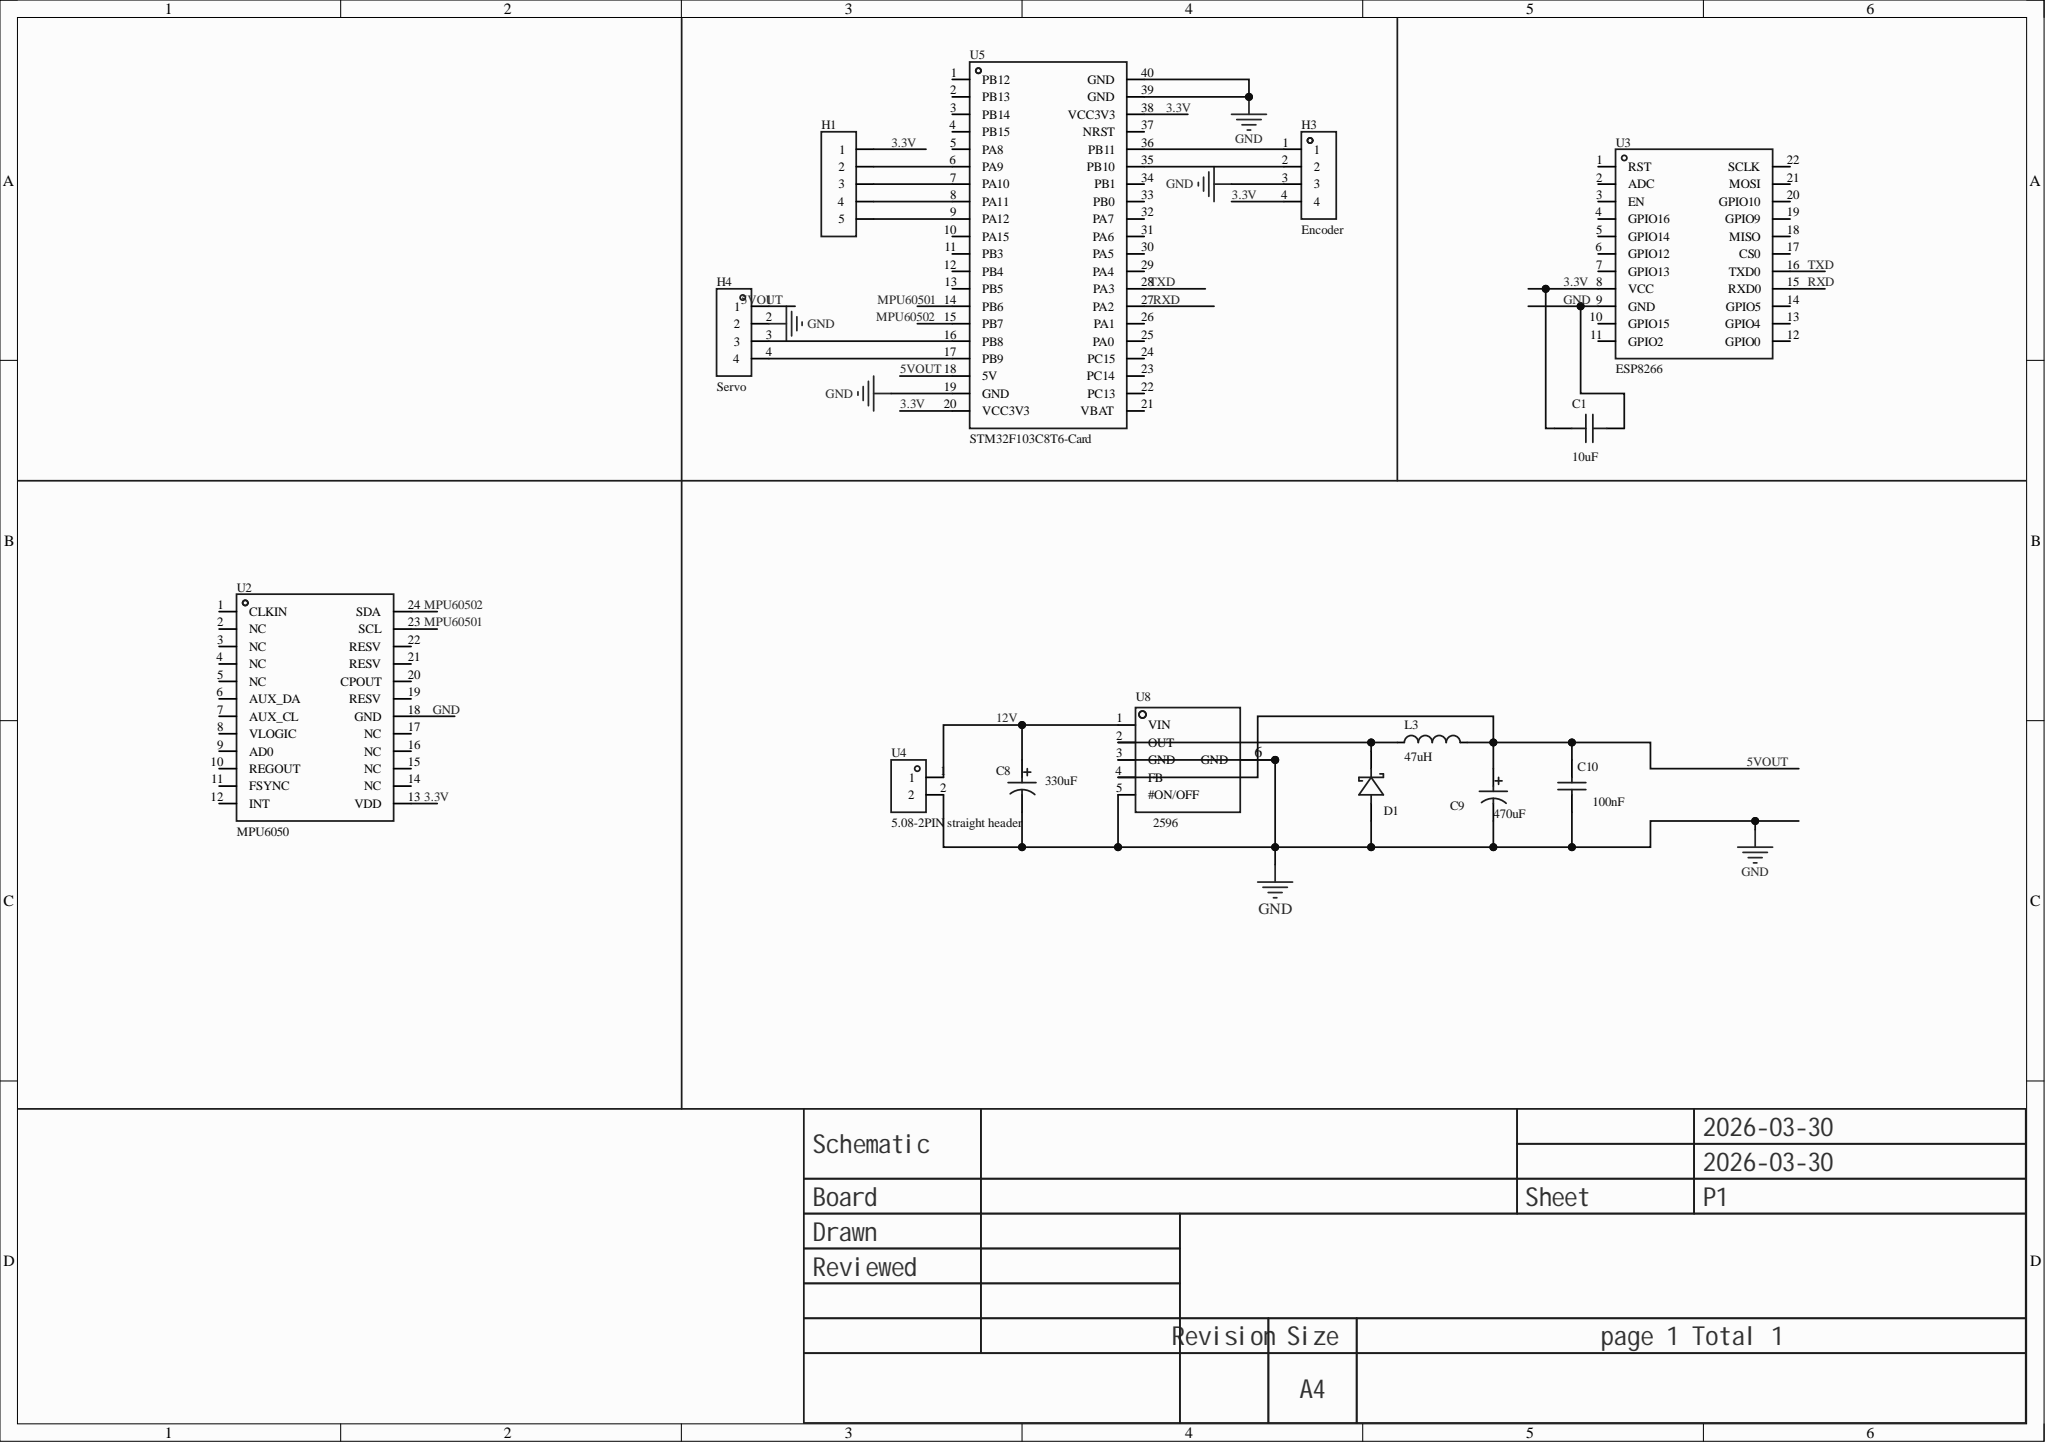Circuit board | Altium Designer | 14 parts | 17 nets
Bill of materials:
Comment,Description,Designator,Footprint,LibRef,Quantity
"10uF","","C1","C0603","CAP_0603","1"
"","Capacitance: 220uF; Tolerance: ±20%; Rated voltage: 35V; Body diameter: 8mm; Body length: 10.5mm; Ripple current: -; ESR: -; Lifetime: 2000hrs@105; Operating temperature: -40~+105;","C8, C9","CAP-SMD_BD8.0-L8.3-W8.3-RD","CS1V221M-CRF10","2"
"","Capacitance: 100nF; Tolerance: ±10%; Rated voltage: 50V; Temperature coefficient: X7R;","C10","C0805","CL21B104KBCNNNC","1"
"","","D1","SMA_L4.3-W2.6-LS5.2-RD","SS34_3","1"
"","","H1","HDR-TH_5P-P2.54-V-F","HDR-F_2.54_1x5P","1"
"Encoder","Pin structure: 1x4P; Pitch: 2.54mm; Row spacing: -; Square/round pins: Square; Mounting: Through-hole; Rows: Single row; Total pins: 4P; Rated current: 3A; Rated voltage: 250V; Mating pin length: 6mm; Housing height: 2.5mm; Tail length: 3mm; Contact material: -; Operating temperature: -40℃~+105℃; Color: Black;","H3","HDR-TH_4P-P2.54-V-M","PZ254V-11-04P","1"
"Servo","Pin structure: 1x4P; Pitch: 2.54mm; Row spacing: -; Square/round pins: Square; Mounting: Through-hole; Rows: Single row; Total pins: 4P; Rated current: 3A; Rated voltage: 250V; Mating pin length: 6mm; Housing height: 2.5mm; Tail length: 3mm; Contact material: -; Operating temperature: -40℃~+105℃; Color: Black;","H4","HDR-TH_4P-P2.54-V-M","PZ254V-11-04P","1"
"","Inductance: 33uH; Tolerance: ±20%; DCR: 270mO;","L3","IND-SMD_L7.0-W6.6","CMLO0630H330MTT","1"
"MPU6050","","U2","QFN-24_L4.0-W4.0-P0.50-BL","MPU6050","1"
"ESP8266","","U3","WIFIM-SMD_ESP-12F-ESP8266MOD","ESP8266","1"
"5.08-2PIN straight header","","U4","HDR-TH_2P-P5.08_C9900004333","5.08-2PIN直针座","1"
"STM32F103C8T6-Card","","U5","CONN-TH_L53.3-W22.9_STM32F103C8T6-CARD","STM32F103C8T6-Card","1"
"LM2596S-5.0","Function type: Step-down; Output type: Fixed; Input voltage: 40V; Output voltage: 5V; Output current (max): 3A;","U8","TO-263-5_L10.2-W8.9-P1.70-BR","LM2596S-5.0_C347421","1"
Netlist (Protel format):
[
C1
C0603
10uF



]
[
C8
CAP-SMD_BD8.0-L8.3-W8.3-RD




]
[
C9
CAP-SMD_BD8.0-L8.3-W8.3-RD




]
[
C10
C0805




]
[
D1
SMA_L4.3-W2.6-LS5.2-RD




]
[
H1
HDR-TH_5P-P2.54-V-F




]
[
H3
HDR-TH_4P-P2.54-V-M
Encoder



]
[
H4
HDR-TH_4P-P2.54-V-M
Servo



]
[
L3
IND-SMD_L7.0-W6.6




]
[
U2
QFN-24_L4.0-W4.0-P0.50-BL
MPU6050



]
[
U3
WIFIM-SMD_ESP-12F-ESP8266MOD
ESP8266



]
[
U4
HDR-TH_2P-P5.08_C9900004333
5.08-2PIN straight header



]
[
U5
CONN-TH_L53.3-W22.9_STM32F103C8T6-CARD
STM32F103C8T6-Card



]
[
U8
TO-263-5_L10.2-W8.9-P1.70-BR
LM2596S-5.0



]
(
TXD
U3-16
U5-28
)
(
RXD
U3-15
U5-27
)
(
NetH4_4
H4-4
U5-17
)
(
NetH4_3
H4-3
U5-16
)
(
NetH3_2
H3-2
U5-35
)
(
NetH3_1
H3-1
U5-36
)
(
NetH1_5
H1-5
U5-9
)
(
NetH1_4
H1-4
U5-8
)
(
NetH1_3
H1-3
U5-7
)
(
NetH1_2
H1-2
U5-6
)
(
NetD1_1
D1-1
L3-1
U8-2
)
(
MPU60502
U2-24
U5-15
)
(
MPU60501
U2-23
U5-14
)
(
GND
C1-2
C8-2
C9-2
C10-2
D1-2
H3-3
H4-2
U2-18
U3-9
U4-2
U5-19
U5-39
U5-40
U8-3
U8-5
U8-6
)
(
12V
C8-1
U4-1
U8-1
)
(
5VOUT
C9-1
C10-1
H4-1
L3-2
U5-18
U8-4
)
(
3.3V
C1-1
H1-1
H3-4
U2-13
U3-8
U5-20
U5-38
)